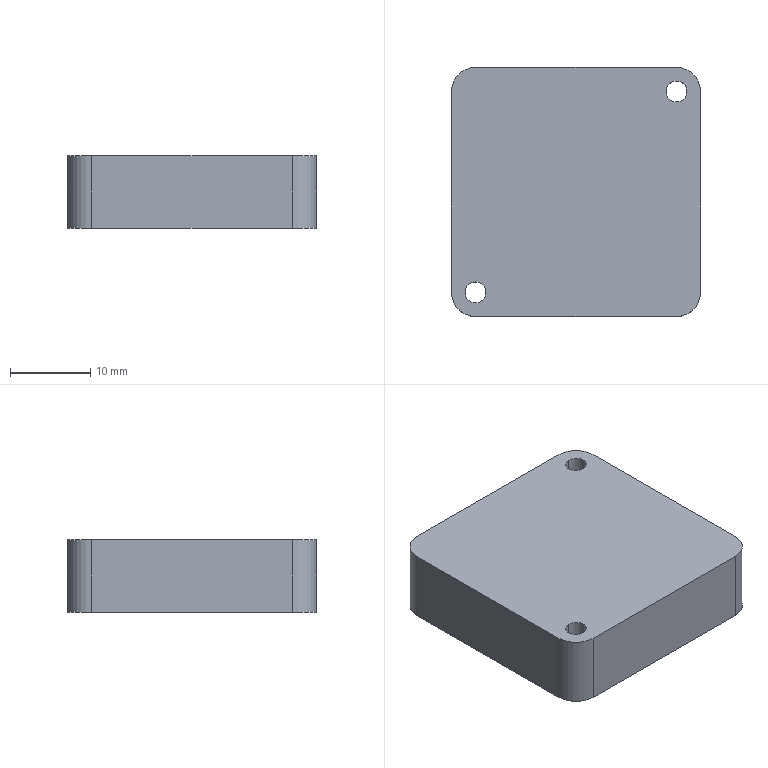NC program | NX | posted with a generic post | part box 31 x 31 x 9 mm
Whole program:
N10 G17 G21 G94 G90
(FLOOR_WALL , TOOL : D63)
N12 T01 M6
N14 G54
N16 G17 G0 G90 X-52. Y0. S6500 M3
N18 G43 Z30. H1
N20 Z3.
N22 G94 G1 Z0. F1250.
N24 X-49.
N26 X49.
N28 X52.
N30 Z3.
N32 G0 Z30.
N34 M5
(DRILLING , TOOL : D6A45)
N36 T07 M6
N38 G54
N40 G17 G0 G90 X-12.5 Y-12.5 S5000 M3
N42 G43 Z30. H7
N44 G94 G81 G98 Z-1.6 F250. R3.
N46 X12.5 Y12.5
N48 G80
N50 G0 X12.5 Y12.5 Z30.
N52 M5
(DRILLING_COPY , TOOL : 2.6ZT)
N54 T12 M6
N56 G54
N58 G17 G0 G90 X-12.5 Y-12.5 S2000 M3
N60 G43 Z30. H12
N62 G94 G83 G98 Z-11.281 F120. Q2. R3.
N64 X12.5 Y12.5
N66 G80
N68 G0 X12.5 Y12.5 Z30.
N70 M5
(ZLEVEL_PROFILE , TOOL : D10)
N72 T10 M6
N74 G54
N76 G17 G0 G90 X20.138 Y-15.227 S9500 M3
N78 G43 Z30. H10
N80 Z1.5
N82 G94 G1 X19.421 Y-16.765 Z1.411 F1000.
N84 X18.249 Y-18.249 Z1.312
N86 X16.765 Y-19.421 Z1.213
N88 X15.05 Y-20.22 Z1.114
N90 X13.198 Y-20.6 Z1.015
N92 X12.5 Z0.978
N94 X-12.5 Z-0.332
N96 X-13.198 Z-0.369
N98 X-15.05 Y-20.22 Z-0.468
N100 X-16.765 Y-19.421 Z-0.567
N102 X-18.249 Y-18.249 Z-0.666
N104 X-19.421 Y-16.765 Z-0.765
N106 X-20.22 Y-15.05 Z-0.864
N108 X-20.6 Y-13.198 Z-0.963
N110 Y-12.5 Z-1.
N112 Y12.5 F2500.
N114 G2 X-12.5 Y20.6 R8.1
N116 G1 X12.5
N118 G2 X20.6 Y12.5 R8.1
N120 G1 Y-12.5
N122 G2 X12.5 Y-20.6 R8.1
N124 G1 X-12.5
N126 G2 X-20.6 Y-12.5 R8.1
N128 G1 Y12.274 Z-1.432
N130 X-20.598 Y12.661 Z-1.439
N132 X-20.581 Y13.048 Z-1.446
N134 X-20.546 Y13.433 Z-1.453
N136 X-20.492 Y13.817 Z-1.459
N138 X-20.42 Y14.197 Z-1.466
N140 X-20.33 Y14.573 Z-1.473
N142 X-20.222 Y14.945 Z-1.48
N144 X-20.097 Y15.311 Z-1.486
N146 X-19.954 Y15.671 Z-1.493
N148 X-19.794 Y16.023 Z-1.5
N150 X-19.617 Y16.368 Z-1.507
N152 X-19.424 Y16.703 Z-1.514
N154 X-19.215 Y17.029 Z-1.52
N156 X-18.991 Y17.345 Z-1.527
N158 X-18.753 Y17.649 Z-1.534
N160 X-18.499 Y17.942 Z-1.541
N162 X-18.233 Y18.223 Z-1.547
N164 X-17.953 Y18.49 Z-1.554
N166 X-17.66 Y18.744 Z-1.561
N168 X-17.356 Y18.983 Z-1.568
N170 X-17.041 Y19.207 Z-1.574
N172 X-16.715 Y19.417 Z-1.581
N174 X-16.38 Y19.61 Z-1.588
N176 X-16.036 Y19.787 Z-1.595
N178 X-15.684 Y19.948 Z-1.601
N180 X-15.324 Y20.092 Z-1.608
N182 X-14.958 Y20.218 Z-1.615
N184 X-14.587 Y20.327 Z-1.622
N186 X-14.211 Y20.417 Z-1.628
N188 X-13.831 Y20.49 Z-1.635
N190 X-13.447 Y20.544 Z-1.642
N192 X-13.062 Y20.58 Z-1.649
N194 X-12.675 Y20.598 Z-1.655
N196 X-12.288 Y20.6 Z-1.662
N198 X7.067 Z-2.
N200 X12.5
N202 G2 X20.6 Y12.5 R8.1
N204 G1 Y-12.5
N206 G2 X12.5 Y-20.6 R8.1
N208 G1 X-12.5
N210 G2 X-20.6 Y-12.5 R8.1
N212 G1 Y12.274 Z-2.432
N214 X-20.598 Y12.661 Z-2.439
N216 X-20.581 Y13.048 Z-2.446
N218 X-20.546 Y13.433 Z-2.453
N220 X-20.492 Y13.817 Z-2.459
N222 X-20.42 Y14.197 Z-2.466
N224 X-20.33 Y14.573 Z-2.473
N226 X-20.222 Y14.945 Z-2.48
N228 X-20.097 Y15.311 Z-2.486
N230 X-19.954 Y15.671 Z-2.493
N232 X-19.794 Y16.023 Z-2.5
N234 X-19.617 Y16.368 Z-2.507
N236 X-19.424 Y16.703 Z-2.514
N238 X-19.215 Y17.029 Z-2.52
N240 X-18.991 Y17.345 Z-2.527
N242 X-18.753 Y17.649 Z-2.534
N244 X-18.499 Y17.942 Z-2.541
N246 X-18.233 Y18.223 Z-2.547
N248 X-17.953 Y18.49 Z-2.554
N250 X-17.66 Y18.744 Z-2.561
N252 X-17.356 Y18.983 Z-2.568
N254 X-17.041 Y19.207 Z-2.574
N256 X-16.715 Y19.417 Z-2.581
N258 X-16.38 Y19.61 Z-2.588
N260 X-16.036 Y19.787 Z-2.595
N262 X-15.684 Y19.948 Z-2.601
N264 X-15.324 Y20.092 Z-2.608
N266 X-14.958 Y20.218 Z-2.615
N268 X-14.587 Y20.327 Z-2.622
N270 X-14.211 Y20.417 Z-2.628
N272 X-13.831 Y20.49 Z-2.635
N274 X-13.447 Y20.544 Z-2.642
N276 X-13.062 Y20.58 Z-2.649
N278 X-12.675 Y20.598 Z-2.655
N280 X-12.288 Y20.6 Z-2.662
N282 X7.067 Z-3.
N284 X12.5
N286 G2 X20.6 Y12.5 R8.1
N288 G1 Y-12.5
N290 G2 X12.5 Y-20.6 R8.1
N292 G1 X-12.5
N294 G2 X-20.6 Y-12.5 R8.1
N296 G1 Y12.274 Z-3.432
N298 X-20.598 Y12.661 Z-3.439
N300 X-20.581 Y13.048 Z-3.446
N302 X-20.546 Y13.433 Z-3.453
N304 X-20.492 Y13.817 Z-3.459
N306 X-20.42 Y14.197 Z-3.466
N308 X-20.33 Y14.573 Z-3.473
N310 X-20.222 Y14.945 Z-3.48
N312 X-20.097 Y15.311 Z-3.486
N314 X-19.954 Y15.671 Z-3.493
N316 X-19.794 Y16.023 Z-3.5
N318 X-19.617 Y16.368 Z-3.507
N320 X-19.424 Y16.703 Z-3.514
N322 X-19.215 Y17.029 Z-3.52
N324 X-18.991 Y17.345 Z-3.527
N326 X-18.753 Y17.649 Z-3.534
N328 X-18.499 Y17.942 Z-3.541
N330 X-18.233 Y18.223 Z-3.547
N332 X-17.953 Y18.49 Z-3.554
N334 X-17.66 Y18.744 Z-3.561
N336 X-17.356 Y18.983 Z-3.568
N338 X-17.041 Y19.207 Z-3.574
N340 X-16.715 Y19.417 Z-3.581
N342 X-16.38 Y19.61 Z-3.588
N344 X-16.036 Y19.787 Z-3.595
N346 X-15.684 Y19.948 Z-3.601
N348 X-15.324 Y20.092 Z-3.608
N350 X-14.958 Y20.218 Z-3.615
N352 X-14.587 Y20.327 Z-3.622
N354 X-14.211 Y20.417 Z-3.628
N356 X-13.831 Y20.49 Z-3.635
N358 X-13.447 Y20.544 Z-3.642
N360 X-13.062 Y20.58 Z-3.649
N362 X-12.675 Y20.598 Z-3.655
N364 X-12.288 Y20.6 Z-3.662
N366 X7.067 Z-4.
N368 X12.5
N370 G2 X20.6 Y12.5 R8.1
N372 G1 Y-12.5
N374 G2 X12.5 Y-20.6 R8.1
N376 G1 X-12.5
N378 G2 X-20.6 Y-12.5 R8.1
N380 G1 Y12.274 Z-4.432
N382 X-20.598 Y12.661 Z-4.439
N384 X-20.581 Y13.048 Z-4.446
N386 X-20.546 Y13.433 Z-4.453
N388 X-20.492 Y13.817 Z-4.459
N390 X-20.42 Y14.197 Z-4.466
N392 X-20.33 Y14.573 Z-4.473
N394 X-20.222 Y14.945 Z-4.48
N396 X-20.097 Y15.311 Z-4.486
N398 X-19.954 Y15.671 Z-4.493
N400 X-19.794 Y16.023 Z-4.5
N402 X-19.617 Y16.368 Z-4.507
N404 X-19.424 Y16.703 Z-4.514
N406 X-19.215 Y17.029 Z-4.52
N408 X-18.991 Y17.345 Z-4.527
N410 X-18.753 Y17.649 Z-4.534
N412 X-18.499 Y17.942 Z-4.541
N414 X-18.233 Y18.223 Z-4.547
N416 X-17.953 Y18.49 Z-4.554
N418 X-17.66 Y18.744 Z-4.561
N420 X-17.356 Y18.983 Z-4.568
N422 X-17.041 Y19.207 Z-4.574
N424 X-16.715 Y19.417 Z-4.581
N426 X-16.38 Y19.61 Z-4.588
N428 X-16.036 Y19.787 Z-4.595
N430 X-15.684 Y19.948 Z-4.601
N432 X-15.324 Y20.092 Z-4.608
N434 X-14.958 Y20.218 Z-4.615
N436 X-14.587 Y20.327 Z-4.622
N438 X-14.211 Y20.417 Z-4.628
N440 X-13.831 Y20.49 Z-4.635
N442 X-13.447 Y20.544 Z-4.642
N444 X-13.062 Y20.58 Z-4.649
N446 X-12.675 Y20.598 Z-4.655
N448 X-12.288 Y20.6 Z-4.662
N450 X7.067 Z-5.
N452 X12.5
N454 G2 X20.6 Y12.5 R8.1
N456 G1 Y-12.5
N458 G2 X12.5 Y-20.6 R8.1
N460 G1 X-12.5
N462 G2 X-20.6 Y-12.5 R8.1
N464 G1 Y12.274 Z-5.432
N466 X-20.598 Y12.661 Z-5.439
N468 X-20.581 Y13.048 Z-5.446
N470 X-20.546 Y13.433 Z-5.453
N472 X-20.492 Y13.817 Z-5.459
N474 X-20.42 Y14.197 Z-5.466
N476 X-20.33 Y14.573 Z-5.473
N478 X-20.222 Y14.945 Z-5.48
N480 X-20.097 Y15.311 Z-5.486
N482 X-19.954 Y15.671 Z-5.493
N484 X-19.794 Y16.023 Z-5.5
N486 X-19.617 Y16.368 Z-5.507
N488 X-19.424 Y16.703 Z-5.514
N490 X-19.215 Y17.029 Z-5.52
N492 X-18.991 Y17.345 Z-5.527
N494 X-18.753 Y17.649 Z-5.534
N496 X-18.499 Y17.942 Z-5.541
N498 X-18.233 Y18.223 Z-5.547
N500 X-17.953 Y18.49 Z-5.554
N502 X-17.66 Y18.744 Z-5.561
N504 X-17.356 Y18.983 Z-5.568
N506 X-17.041 Y19.207 Z-5.574
N508 X-16.715 Y19.417 Z-5.581
N510 X-16.38 Y19.61 Z-5.588
N512 X-16.036 Y19.787 Z-5.595
N514 X-15.684 Y19.948 Z-5.601
N516 X-15.324 Y20.092 Z-5.608
N518 X-14.958 Y20.218 Z-5.615
N520 X-14.587 Y20.327 Z-5.622
N522 X-14.211 Y20.417 Z-5.628
N524 X-13.831 Y20.49 Z-5.635
N526 X-13.447 Y20.544 Z-5.642
N528 X-13.062 Y20.58 Z-5.649
N530 X-12.675 Y20.598 Z-5.655
N532 X-12.288 Y20.6 Z-5.662
N534 X7.067 Z-6.
N536 X12.5
N538 G2 X20.6 Y12.5 R8.1
N540 G1 Y-12.5
N542 G2 X12.5 Y-20.6 R8.1
N544 G1 X-12.5
N546 G2 X-20.6 Y-12.5 R8.1
N548 G1 Y12.274 Z-6.432
N550 X-20.598 Y12.661 Z-6.439
N552 X-20.581 Y13.048 Z-6.446
N554 X-20.546 Y13.433 Z-6.453
N556 X-20.492 Y13.817 Z-6.459
N558 X-20.42 Y14.197 Z-6.466
N560 X-20.33 Y14.573 Z-6.473
N562 X-20.222 Y14.945 Z-6.48
N564 X-20.097 Y15.311 Z-6.486
N566 X-19.954 Y15.671 Z-6.493
N568 X-19.794 Y16.023 Z-6.5
N570 X-19.617 Y16.368 Z-6.507
N572 X-19.424 Y16.703 Z-6.514
N574 X-19.215 Y17.029 Z-6.52
N576 X-18.991 Y17.345 Z-6.527
N578 X-18.753 Y17.649 Z-6.534
N580 X-18.499 Y17.942 Z-6.541
N582 X-18.233 Y18.223 Z-6.547
N584 X-17.953 Y18.49 Z-6.554
N586 X-17.66 Y18.744 Z-6.561
N588 X-17.356 Y18.983 Z-6.568
N590 X-17.041 Y19.207 Z-6.574
N592 X-16.715 Y19.417 Z-6.581
N594 X-16.38 Y19.61 Z-6.588
N596 X-16.036 Y19.787 Z-6.595
N598 X-15.684 Y19.948 Z-6.601
N600 X-15.324 Y20.092 Z-6.608
N602 X-14.958 Y20.218 Z-6.615
N604 X-14.587 Y20.327 Z-6.622
N606 X-14.211 Y20.417 Z-6.628
N608 X-13.831 Y20.49 Z-6.635
N610 X-13.447 Y20.544 Z-6.642
N612 X-13.062 Y20.58 Z-6.649
N614 X-12.675 Y20.598 Z-6.655
N616 X-12.288 Y20.6 Z-6.662
N618 X7.067 Z-7.
N620 X12.5
N622 G2 X20.6 Y12.5 R8.1
N624 G1 Y-12.5
N626 G2 X12.5 Y-20.6 R8.1
N628 G1 X-12.5
N630 G2 X-20.6 Y-12.5 R8.1
N632 G1 Y12.274 Z-7.432
N634 X-20.598 Y12.661 Z-7.439
N636 X-20.581 Y13.048 Z-7.446
N638 X-20.546 Y13.433 Z-7.453
N640 X-20.492 Y13.817 Z-7.459
N642 X-20.42 Y14.197 Z-7.466
N644 X-20.33 Y14.573 Z-7.473
N646 X-20.222 Y14.945 Z-7.48
N648 X-20.097 Y15.311 Z-7.486
N650 X-19.954 Y15.671 Z-7.493
N652 X-19.794 Y16.023 Z-7.5
N654 X-19.617 Y16.368 Z-7.507
N656 X-19.424 Y16.703 Z-7.514
N658 X-19.215 Y17.029 Z-7.52
N660 X-18.991 Y17.345 Z-7.527
N662 X-18.753 Y17.649 Z-7.534
N664 X-18.499 Y17.942 Z-7.541
N666 X-18.233 Y18.223 Z-7.547
N668 X-17.953 Y18.49 Z-7.554
N670 X-17.66 Y18.744 Z-7.561
N672 X-17.356 Y18.983 Z-7.568
N674 X-17.041 Y19.207 Z-7.574
N676 X-16.715 Y19.417 Z-7.581
N678 X-16.38 Y19.61 Z-7.588
N680 X-16.036 Y19.787 Z-7.595
N682 X-15.684 Y19.948 Z-7.601
N684 X-15.324 Y20.092 Z-7.608
N686 X-14.958 Y20.218 Z-7.615
N688 X-14.587 Y20.327 Z-7.622
N690 X-14.211 Y20.417 Z-7.628
N692 X-13.831 Y20.49 Z-7.635
N694 X-13.447 Y20.544 Z-7.642
N696 X-13.062 Y20.58 Z-7.649
N698 X-12.675 Y20.598 Z-7.655
N700 X-12.288 Y20.6 Z-7.662
N702 X7.067 Z-8.
N704 X12.5
N706 G2 X20.6 Y12.5 R8.1
N708 G1 Y-12.5
N710 G2 X12.5 Y-20.6 R8.1
N712 G1 X-12.5
N714 G2 X-20.6 Y-12.5 R8.1
N716 G1 Y12.274 Z-8.432
N718 X-20.598 Y12.661 Z-8.439
N720 X-20.581 Y13.048 Z-8.446
N722 X-20.546 Y13.433 Z-8.453
N724 X-20.492 Y13.817 Z-8.459
N726 X-20.42 Y14.197 Z-8.466
N728 X-20.33 Y14.573 Z-8.473
N730 X-20.222 Y14.945 Z-8.48
N732 X-20.097 Y15.311 Z-8.486
N734 X-19.954 Y15.671 Z-8.493
N736 X-19.794 Y16.023 Z-8.5
N738 X-19.617 Y16.368 Z-8.507
N740 X-19.424 Y16.703 Z-8.514
N742 X-19.215 Y17.029 Z-8.52
N744 X-18.991 Y17.345 Z-8.527
N746 X-18.753 Y17.649 Z-8.534
N748 X-18.499 Y17.942 Z-8.541
N750 X-18.233 Y18.223 Z-8.547
N752 X-17.953 Y18.49 Z-8.554
N754 X-17.66 Y18.744 Z-8.561
N756 X-17.356 Y18.983 Z-8.568
N758 X-17.041 Y19.207 Z-8.574
N760 X-16.715 Y19.417 Z-8.581
N762 X-16.38 Y19.61 Z-8.588
N764 X-16.036 Y19.787 Z-8.595
N766 X-15.684 Y19.948 Z-8.601
N768 X-15.324 Y20.092 Z-8.608
N770 X-14.958 Y20.218 Z-8.615
N772 X-14.587 Y20.327 Z-8.622
N774 X-14.211 Y20.417 Z-8.628
N776 X-13.831 Y20.49 Z-8.635
N778 X-13.447 Y20.544 Z-8.642
N780 X-13.062 Y20.58 Z-8.649
N782 X-12.675 Y20.598 Z-8.655
N784 X-12.288 Y20.6 Z-8.662
N786 X7.067 Z-9.
N788 X12.5
N790 G2 X20.6 Y12.5 R8.1
N792 G1 Y-12.5
N794 G2 X12.5 Y-20.6 R8.1
N796 G1 X-12.5
N798 G2 X-20.6 Y-12.5 R8.1
N800 G1 Y12.5
N802 G2 X-12.5 Y20.6 R8.1
N804 G1 X7.067
N806 Z-7.5
N808 G0 Z30.
(ZLEVEL_PROFILE_COPY , TOOL : D10)
N810 X-22.362 Y-14.153
N812 Z-7.5
N814 G1 Z-9. F1000.
N816 X-21. Y-13.366
N818 G3 X-20.5 Y-12.5 R1.
N820 G1 Y12.5 F1200.
N822 G2 X-12.5 Y20.5 R8.
N824 G1 X12.5
N826 G2 X20.5 Y12.5 R8.
N828 G1 Y-12.5
N830 G2 X12.5 Y-20.5 R8.
N832 G1 X-12.5
N834 G2 X-20.5 Y-12.5 R8.
N836 G3 X-21. Y-11.634 R1.
N838 G1 X-22.5 Y-10.768
N840 Z-7.5
N842 G0 Z30.
N844 M5
N846 M2